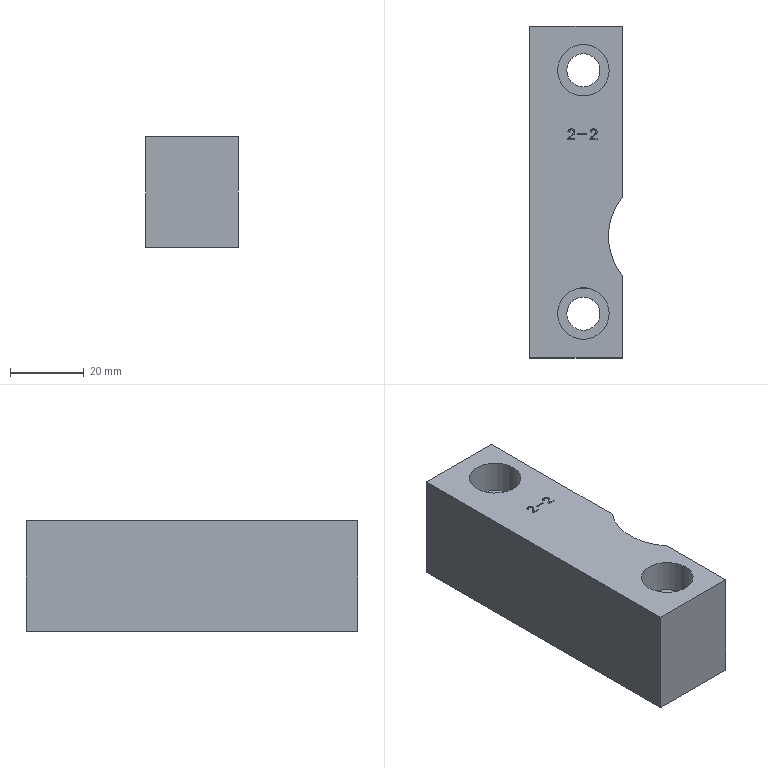Part | STEP file | solid 19 | 1 solid | 33 faces | box 25 x 90 x 30 mm | volume 60451 mm3 | plane 24 | cylinder 5 | other 4 | commonest cylinder face diameters 9 x2 14 x2 34 x1